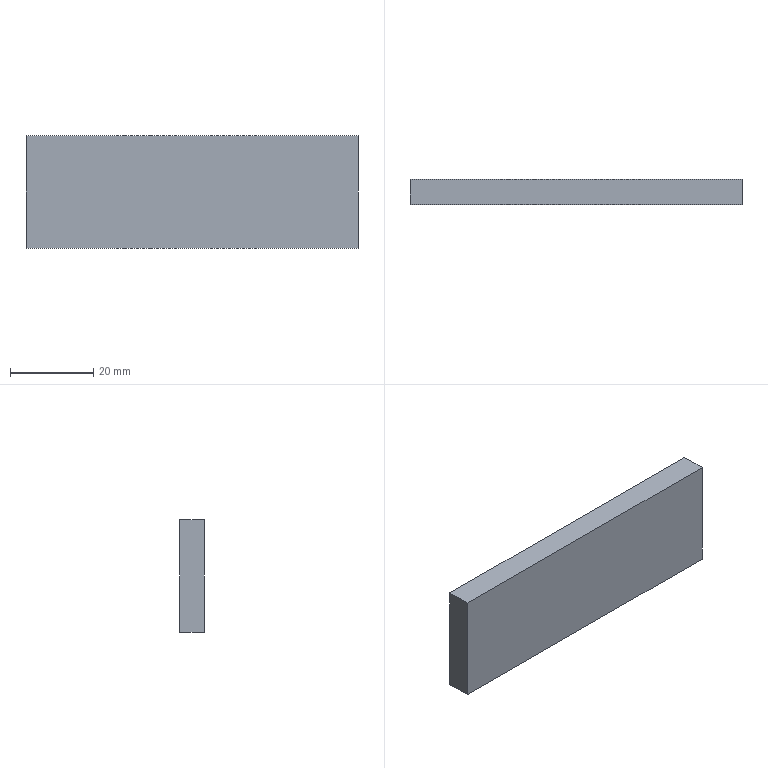Part | STEP file | Positioning_id2314_x_t | 1 solid | 6 faces | box 80 x 6 x 27 mm | volume 12960 mm3 | plane 6
STEP:
#1=CARTESIAN_POINT('',(0.,0.,0.));
#2=DIRECTION('',(0.,0.,1.));
#3=DIRECTION('',(1.,0.,0.));
#4=AXIS2_PLACEMENT_3D('',#1,#2,#3);
#5=CARTESIAN_POINT('',(-923.002,297.,225.532));
#6=VERTEX_POINT('',#5);
#7=CARTESIAN_POINT('',(-923.002,303.,225.532));
#8=VERTEX_POINT('',#7);
#9=CARTESIAN_POINT('',(-923.002,297.,225.532));
#10=DIRECTION('',(0.,1.,0.));
#11=VECTOR('',#10,1.);
#12=LINE('',#9,#11);
#13=CARTESIAN_POINT('',(-923.002,268.,225.532));
#14=DIRECTION('',(0.,0.,-1.));
#15=DIRECTION('',(-1.,0.,0.));
#16=AXIS2_PLACEMENT_3D('',#13,#14,#15);
#17=PLANE('',#16);
#18=CARTESIAN_POINT('',(0.,29.));
#19=DIRECTION('',(0.,1.));
#20=VECTOR('',#19,1.);
#21=LINE('',#18,#20);
#22=(GEOMETRIC_REPRESENTATION_CONTEXT(2)PARAMETRIC_REPRESENTATION_CONTEXT()REPRESENTATION_CONTEXT('',''));
#23=DEFINITIONAL_REPRESENTATION('',(#21),#22);
#24=PCURVE('',#17,#23);
#25=CARTESIAN_POINT('',(-923.002,298.5,217.532));
#26=DIRECTION('',(1.,0.,0.));
#27=DIRECTION('',(0.,1.,0.));
#28=AXIS2_PLACEMENT_3D('',#25,#26,#27);
#29=PLANE('',#28);
#30=CARTESIAN_POINT('',(-1.5,8.));
#31=DIRECTION('',(1.,0.));
#32=VECTOR('',#31,1.);
#33=LINE('',#30,#32);
#34=(GEOMETRIC_REPRESENTATION_CONTEXT(2)PARAMETRIC_REPRESENTATION_CONTEXT()REPRESENTATION_CONTEXT('',''));
#35=DEFINITIONAL_REPRESENTATION('',(#33),#34);
#36=PCURVE('',#29,#35);
#37=SURFACE_CURVE('',#12,(#24,#36),.PCURVE_S1.);
#38=EDGE_CURVE('',#6,#8,#37,.T.);
#39=ORIENTED_EDGE('',*,*,#38,.T.);
#40=CARTESIAN_POINT('',(-1003.002,303.,225.532));
#41=VERTEX_POINT('',#40);
#42=CARTESIAN_POINT('',(-923.002,303.,225.532));
#43=DIRECTION('',(-1.,0.,0.));
#44=VECTOR('',#43,1.);
#45=LINE('',#42,#44);
#46=CARTESIAN_POINT('',(0.,35.));
#47=DIRECTION('',(1.,0.));
#48=VECTOR('',#47,1.);
#49=LINE('',#46,#48);
#50=(GEOMETRIC_REPRESENTATION_CONTEXT(2)PARAMETRIC_REPRESENTATION_CONTEXT()REPRESENTATION_CONTEXT('',''));
#51=DEFINITIONAL_REPRESENTATION('',(#49),#50);
#52=PCURVE('',#17,#51);
#53=CARTESIAN_POINT('',(-1003.002,303.,217.532));
#54=DIRECTION('',(0.,1.,0.));
#55=DIRECTION('',(-1.,0.,0.));
#56=AXIS2_PLACEMENT_3D('',#53,#54,#55);
#57=PLANE('',#56);
#58=CARTESIAN_POINT('',(-80.,8.));
#59=DIRECTION('',(1.,0.));
#60=VECTOR('',#59,1.);
#61=LINE('',#58,#60);
#62=(GEOMETRIC_REPRESENTATION_CONTEXT(2)PARAMETRIC_REPRESENTATION_CONTEXT()REPRESENTATION_CONTEXT('',''));
#63=DEFINITIONAL_REPRESENTATION('',(#61),#62);
#64=PCURVE('',#57,#63);
#65=SURFACE_CURVE('',#45,(#52,#64),.PCURVE_S1.);
#66=EDGE_CURVE('',#8,#41,#65,.T.);
#67=ORIENTED_EDGE('',*,*,#66,.T.);
#68=CARTESIAN_POINT('',(-1003.002,297.,225.532));
#69=VERTEX_POINT('',#68);
#70=CARTESIAN_POINT('',(-1003.002,303.,225.532));
#71=DIRECTION('',(0.,-1.,0.));
#72=VECTOR('',#71,1.);
#73=LINE('',#70,#72);
#74=CARTESIAN_POINT('',(80.,35.));
#75=DIRECTION('',(0.,-1.));
#76=VECTOR('',#75,1.);
#77=LINE('',#74,#76);
#78=(GEOMETRIC_REPRESENTATION_CONTEXT(2)PARAMETRIC_REPRESENTATION_CONTEXT()REPRESENTATION_CONTEXT('',''));
#79=DEFINITIONAL_REPRESENTATION('',(#77),#78);
#80=PCURVE('',#17,#79);
#81=CARTESIAN_POINT('',(-1003.002,298.5,217.532));
#82=DIRECTION('',(-1.,0.,0.));
#83=DIRECTION('',(0.,-1.,0.));
#84=AXIS2_PLACEMENT_3D('',#81,#82,#83);
#85=PLANE('',#84);
#86=CARTESIAN_POINT('',(-4.5,8.));
#87=DIRECTION('',(1.,0.));
#88=VECTOR('',#87,1.);
#89=LINE('',#86,#88);
#90=(GEOMETRIC_REPRESENTATION_CONTEXT(2)PARAMETRIC_REPRESENTATION_CONTEXT()REPRESENTATION_CONTEXT('',''));
#91=DEFINITIONAL_REPRESENTATION('',(#89),#90);
#92=PCURVE('',#85,#91);
#93=SURFACE_CURVE('',#73,(#80,#92),.PCURVE_S1.);
#94=EDGE_CURVE('',#41,#69,#93,.T.);
#95=ORIENTED_EDGE('',*,*,#94,.T.);
#96=CARTESIAN_POINT('',(-1003.002,297.,225.532));
#97=DIRECTION('',(1.,0.,0.));
#98=VECTOR('',#97,1.);
#99=LINE('',#96,#98);
#100=CARTESIAN_POINT('',(80.,29.));
#101=DIRECTION('',(-1.,0.));
#102=VECTOR('',#101,1.);
#103=LINE('',#100,#102);
#104=(GEOMETRIC_REPRESENTATION_CONTEXT(2)PARAMETRIC_REPRESENTATION_CONTEXT()REPRESENTATION_CONTEXT('',''));
#105=DEFINITIONAL_REPRESENTATION('',(#103),#104);
#106=PCURVE('',#17,#105);
#107=CARTESIAN_POINT('',(-1003.002,297.,217.532));
#108=DIRECTION('',(0.,-1.,0.));
#109=DIRECTION('',(1.,0.,0.));
#110=AXIS2_PLACEMENT_3D('',#107,#108,#109);
#111=PLANE('',#110);
#112=CARTESIAN_POINT('',(0.,8.));
#113=DIRECTION('',(1.,0.));
#114=VECTOR('',#113,1.);
#115=LINE('',#112,#114);
#116=(GEOMETRIC_REPRESENTATION_CONTEXT(2)PARAMETRIC_REPRESENTATION_CONTEXT()REPRESENTATION_CONTEXT('',''));
#117=DEFINITIONAL_REPRESENTATION('',(#115),#116);
#118=PCURVE('',#111,#117);
#119=SURFACE_CURVE('',#99,(#106,#118),.PCURVE_S1.);
#120=EDGE_CURVE('',#69,#6,#119,.T.);
#121=ORIENTED_EDGE('',*,*,#120,.T.);
#122=EDGE_LOOP('',(#39,#67,#95,#121));
#123=FACE_BOUND('',#122,.T.);
#124=ADVANCED_FACE('',(#123),#17,.F.);
#125=ORIENTED_EDGE('',*,*,#120,.F.);
#126=CARTESIAN_POINT('',(-1003.002,297.,198.532));
#127=VERTEX_POINT('',#126);
#128=CARTESIAN_POINT('',(-1003.002,297.,225.532));
#129=DIRECTION('',(0.,0.,-1.));
#130=VECTOR('',#129,1.);
#131=LINE('',#128,#130);
#132=CARTESIAN_POINT('',(0.,8.));
#133=DIRECTION('',(0.,-1.));
#134=VECTOR('',#133,1.);
#135=LINE('',#132,#134);
#136=(GEOMETRIC_REPRESENTATION_CONTEXT(2)PARAMETRIC_REPRESENTATION_CONTEXT()REPRESENTATION_CONTEXT('',''));
#137=DEFINITIONAL_REPRESENTATION('',(#135),#136);
#138=PCURVE('',#111,#137);
#139=CARTESIAN_POINT('',(1.5,8.));
#140=DIRECTION('',(0.,-1.));
#141=VECTOR('',#140,1.);
#142=LINE('',#139,#141);
#143=(GEOMETRIC_REPRESENTATION_CONTEXT(2)PARAMETRIC_REPRESENTATION_CONTEXT()REPRESENTATION_CONTEXT('',''));
#144=DEFINITIONAL_REPRESENTATION('',(#142),#143);
#145=PCURVE('',#85,#144);
#146=SURFACE_CURVE('',#131,(#138,#145),.PCURVE_S1.);
#147=EDGE_CURVE('',#69,#127,#146,.T.);
#148=ORIENTED_EDGE('',*,*,#147,.T.);
#149=CARTESIAN_POINT('',(-923.002,297.,198.532));
#150=VERTEX_POINT('',#149);
#151=CARTESIAN_POINT('',(-1003.002,297.,198.532));
#152=DIRECTION('',(1.,0.,0.));
#153=VECTOR('',#152,1.);
#154=LINE('',#151,#153);
#155=CARTESIAN_POINT('',(0.,-19.));
#156=DIRECTION('',(1.,0.));
#157=VECTOR('',#156,1.);
#158=LINE('',#155,#157);
#159=(GEOMETRIC_REPRESENTATION_CONTEXT(2)PARAMETRIC_REPRESENTATION_CONTEXT()REPRESENTATION_CONTEXT('',''));
#160=DEFINITIONAL_REPRESENTATION('',(#158),#159);
#161=PCURVE('',#111,#160);
#162=CARTESIAN_POINT('',(-1003.002,298.5,198.532));
#163=DIRECTION('',(0.,0.,-1.));
#164=DIRECTION('',(-1.,0.,0.));
#165=AXIS2_PLACEMENT_3D('',#162,#163,#164);
#166=PLANE('',#165);
#167=CARTESIAN_POINT('',(0.,-1.5));
#168=DIRECTION('',(-1.,0.));
#169=VECTOR('',#168,1.);
#170=LINE('',#167,#169);
#171=(GEOMETRIC_REPRESENTATION_CONTEXT(2)PARAMETRIC_REPRESENTATION_CONTEXT()REPRESENTATION_CONTEXT('',''));
#172=DEFINITIONAL_REPRESENTATION('',(#170),#171);
#173=PCURVE('',#166,#172);
#174=SURFACE_CURVE('',#154,(#161,#173),.PCURVE_S1.);
#175=EDGE_CURVE('',#127,#150,#174,.T.);
#176=ORIENTED_EDGE('',*,*,#175,.T.);
#177=CARTESIAN_POINT('',(-923.002,297.,198.532));
#178=DIRECTION('',(0.,0.,1.));
#179=VECTOR('',#178,1.);
#180=LINE('',#177,#179);
#181=CARTESIAN_POINT('',(80.,-19.));
#182=DIRECTION('',(0.,1.));
#183=VECTOR('',#182,1.);
#184=LINE('',#181,#183);
#185=(GEOMETRIC_REPRESENTATION_CONTEXT(2)PARAMETRIC_REPRESENTATION_CONTEXT()REPRESENTATION_CONTEXT('',''));
#186=DEFINITIONAL_REPRESENTATION('',(#184),#185);
#187=PCURVE('',#111,#186);
#188=CARTESIAN_POINT('',(-1.5,-19.));
#189=DIRECTION('',(0.,1.));
#190=VECTOR('',#189,1.);
#191=LINE('',#188,#190);
#192=(GEOMETRIC_REPRESENTATION_CONTEXT(2)PARAMETRIC_REPRESENTATION_CONTEXT()REPRESENTATION_CONTEXT('',''));
#193=DEFINITIONAL_REPRESENTATION('',(#191),#192);
#194=PCURVE('',#29,#193);
#195=SURFACE_CURVE('',#180,(#187,#194),.PCURVE_S1.);
#196=EDGE_CURVE('',#150,#6,#195,.T.);
#197=ORIENTED_EDGE('',*,*,#196,.T.);
#198=EDGE_LOOP('',(#125,#148,#176,#197));
#199=FACE_BOUND('',#198,.T.);
#200=ADVANCED_FACE('',(#199),#111,.T.);
#201=ORIENTED_EDGE('',*,*,#94,.F.);
#202=CARTESIAN_POINT('',(-1003.002,303.,198.532));
#203=VERTEX_POINT('',#202);
#204=CARTESIAN_POINT('',(-1003.002,303.,198.532));
#205=DIRECTION('',(0.,0.,1.));
#206=VECTOR('',#205,1.);
#207=LINE('',#204,#206);
#208=CARTESIAN_POINT('',(-4.5,-19.));
#209=DIRECTION('',(0.,1.));
#210=VECTOR('',#209,1.);
#211=LINE('',#208,#210);
#212=(GEOMETRIC_REPRESENTATION_CONTEXT(2)PARAMETRIC_REPRESENTATION_CONTEXT()REPRESENTATION_CONTEXT('',''));
#213=DEFINITIONAL_REPRESENTATION('',(#211),#212);
#214=PCURVE('',#85,#213);
#215=CARTESIAN_POINT('',(0.,-19.));
#216=DIRECTION('',(0.,1.));
#217=VECTOR('',#216,1.);
#218=LINE('',#215,#217);
#219=(GEOMETRIC_REPRESENTATION_CONTEXT(2)PARAMETRIC_REPRESENTATION_CONTEXT()REPRESENTATION_CONTEXT('',''));
#220=DEFINITIONAL_REPRESENTATION('',(#218),#219);
#221=PCURVE('',#57,#220);
#222=SURFACE_CURVE('',#207,(#214,#221),.PCURVE_S1.);
#223=EDGE_CURVE('',#203,#41,#222,.T.);
#224=ORIENTED_EDGE('',*,*,#223,.F.);
#225=CARTESIAN_POINT('',(-1003.002,297.,198.532));
#226=DIRECTION('',(0.,1.,0.));
#227=VECTOR('',#226,1.);
#228=LINE('',#225,#227);
#229=CARTESIAN_POINT('',(1.5,-19.));
#230=DIRECTION('',(-1.,0.));
#231=VECTOR('',#230,1.);
#232=LINE('',#229,#231);
#233=(GEOMETRIC_REPRESENTATION_CONTEXT(2)PARAMETRIC_REPRESENTATION_CONTEXT()REPRESENTATION_CONTEXT('',''));
#234=DEFINITIONAL_REPRESENTATION('',(#232),#233);
#235=PCURVE('',#85,#234);
#236=CARTESIAN_POINT('',(0.,-1.5));
#237=DIRECTION('',(0.,1.));
#238=VECTOR('',#237,1.);
#239=LINE('',#236,#238);
#240=(GEOMETRIC_REPRESENTATION_CONTEXT(2)PARAMETRIC_REPRESENTATION_CONTEXT()REPRESENTATION_CONTEXT('',''));
#241=DEFINITIONAL_REPRESENTATION('',(#239),#240);
#242=PCURVE('',#166,#241);
#243=SURFACE_CURVE('',#228,(#235,#242),.PCURVE_S1.);
#244=EDGE_CURVE('',#127,#203,#243,.T.);
#245=ORIENTED_EDGE('',*,*,#244,.F.);
#246=ORIENTED_EDGE('',*,*,#147,.F.);
#247=EDGE_LOOP('',(#201,#224,#245,#246));
#248=FACE_BOUND('',#247,.T.);
#249=ADVANCED_FACE('',(#248),#85,.T.);
#250=CARTESIAN_POINT('',(-923.002,303.,198.532));
#251=VERTEX_POINT('',#250);
#252=CARTESIAN_POINT('',(-1003.002,303.,198.532));
#253=DIRECTION('',(1.,0.,0.));
#254=VECTOR('',#253,1.);
#255=LINE('',#252,#254);
#256=CARTESIAN_POINT('',(0.,4.5));
#257=DIRECTION('',(-1.,0.));
#258=VECTOR('',#257,1.);
#259=LINE('',#256,#258);
#260=(GEOMETRIC_REPRESENTATION_CONTEXT(2)PARAMETRIC_REPRESENTATION_CONTEXT()REPRESENTATION_CONTEXT('',''));
#261=DEFINITIONAL_REPRESENTATION('',(#259),#260);
#262=PCURVE('',#166,#261);
#263=CARTESIAN_POINT('',(0.,-19.));
#264=DIRECTION('',(-1.,0.));
#265=VECTOR('',#264,1.);
#266=LINE('',#263,#265);
#267=(GEOMETRIC_REPRESENTATION_CONTEXT(2)PARAMETRIC_REPRESENTATION_CONTEXT()REPRESENTATION_CONTEXT('',''));
#268=DEFINITIONAL_REPRESENTATION('',(#266),#267);
#269=PCURVE('',#57,#268);
#270=SURFACE_CURVE('',#255,(#262,#269),.PCURVE_S1.);
#271=EDGE_CURVE('',#203,#251,#270,.T.);
#272=ORIENTED_EDGE('',*,*,#271,.T.);
#273=CARTESIAN_POINT('',(-923.002,303.,198.532));
#274=DIRECTION('',(0.,-1.,0.));
#275=VECTOR('',#274,1.);
#276=LINE('',#273,#275);
#277=CARTESIAN_POINT('',(-80.,4.5));
#278=DIRECTION('',(0.,-1.));
#279=VECTOR('',#278,1.);
#280=LINE('',#277,#279);
#281=(GEOMETRIC_REPRESENTATION_CONTEXT(2)PARAMETRIC_REPRESENTATION_CONTEXT()REPRESENTATION_CONTEXT('',''));
#282=DEFINITIONAL_REPRESENTATION('',(#280),#281);
#283=PCURVE('',#166,#282);
#284=CARTESIAN_POINT('',(4.5,-19.));
#285=DIRECTION('',(-1.,0.));
#286=VECTOR('',#285,1.);
#287=LINE('',#284,#286);
#288=(GEOMETRIC_REPRESENTATION_CONTEXT(2)PARAMETRIC_REPRESENTATION_CONTEXT()REPRESENTATION_CONTEXT('',''));
#289=DEFINITIONAL_REPRESENTATION('',(#287),#288);
#290=PCURVE('',#29,#289);
#291=SURFACE_CURVE('',#276,(#283,#290),.PCURVE_S1.);
#292=EDGE_CURVE('',#251,#150,#291,.T.);
#293=ORIENTED_EDGE('',*,*,#292,.T.);
#294=ORIENTED_EDGE('',*,*,#175,.F.);
#295=ORIENTED_EDGE('',*,*,#244,.T.);
#296=EDGE_LOOP('',(#272,#293,#294,#295));
#297=FACE_BOUND('',#296,.T.);
#298=ADVANCED_FACE('',(#297),#166,.T.);
#299=ORIENTED_EDGE('',*,*,#66,.F.);
#300=CARTESIAN_POINT('',(-923.002,303.,225.532));
#301=DIRECTION('',(0.,0.,-1.));
#302=VECTOR('',#301,1.);
#303=LINE('',#300,#302);
#304=CARTESIAN_POINT('',(-80.,8.));
#305=DIRECTION('',(0.,-1.));
#306=VECTOR('',#305,1.);
#307=LINE('',#304,#306);
#308=(GEOMETRIC_REPRESENTATION_CONTEXT(2)PARAMETRIC_REPRESENTATION_CONTEXT()REPRESENTATION_CONTEXT('',''));
#309=DEFINITIONAL_REPRESENTATION('',(#307),#308);
#310=PCURVE('',#57,#309);
#311=CARTESIAN_POINT('',(4.5,8.));
#312=DIRECTION('',(0.,-1.));
#313=VECTOR('',#312,1.);
#314=LINE('',#311,#313);
#315=(GEOMETRIC_REPRESENTATION_CONTEXT(2)PARAMETRIC_REPRESENTATION_CONTEXT()REPRESENTATION_CONTEXT('',''));
#316=DEFINITIONAL_REPRESENTATION('',(#314),#315);
#317=PCURVE('',#29,#316);
#318=SURFACE_CURVE('',#303,(#310,#317),.PCURVE_S1.);
#319=EDGE_CURVE('',#8,#251,#318,.T.);
#320=ORIENTED_EDGE('',*,*,#319,.T.);
#321=ORIENTED_EDGE('',*,*,#271,.F.);
#322=ORIENTED_EDGE('',*,*,#223,.T.);
#323=EDGE_LOOP('',(#299,#320,#321,#322));
#324=FACE_BOUND('',#323,.T.);
#325=ADVANCED_FACE('',(#324),#57,.T.);
#326=ORIENTED_EDGE('',*,*,#38,.F.);
#327=ORIENTED_EDGE('',*,*,#196,.F.);
#328=ORIENTED_EDGE('',*,*,#292,.F.);
#329=ORIENTED_EDGE('',*,*,#319,.F.);
#330=EDGE_LOOP('',(#326,#327,#328,#329));
#331=FACE_BOUND('',#330,.T.);
#332=ADVANCED_FACE('',(#331),#29,.T.);
#333=CLOSED_SHELL('',(#124,#200,#249,#298,#325,#332));
#334=MANIFOLD_SOLID_BREP('',#333);
#335=(LENGTH_UNIT()NAMED_UNIT(*)SI_UNIT(.MILLI.,.METRE.));
#336=UNCERTAINTY_MEASURE_WITH_UNIT(LENGTH_MEASURE(0.0000001),#335,'','');
#337=(NAMED_UNIT(*)PLANE_ANGLE_UNIT()SI_UNIT($,.RADIAN.));
#338=(NAMED_UNIT(*)SI_UNIT($,.STERADIAN.)SOLID_ANGLE_UNIT());
#339=(GEOMETRIC_REPRESENTATION_CONTEXT(3)GLOBAL_UNCERTAINTY_ASSIGNED_CONTEXT((#336))GLOBAL_UNIT_ASSIGNED_CONTEXT((#335,#337,#338))REPRESENTATION_CONTEXT('',''));
#340=ADVANCED_BREP_SHAPE_REPRESENTATION('',(#4,#334),#339);